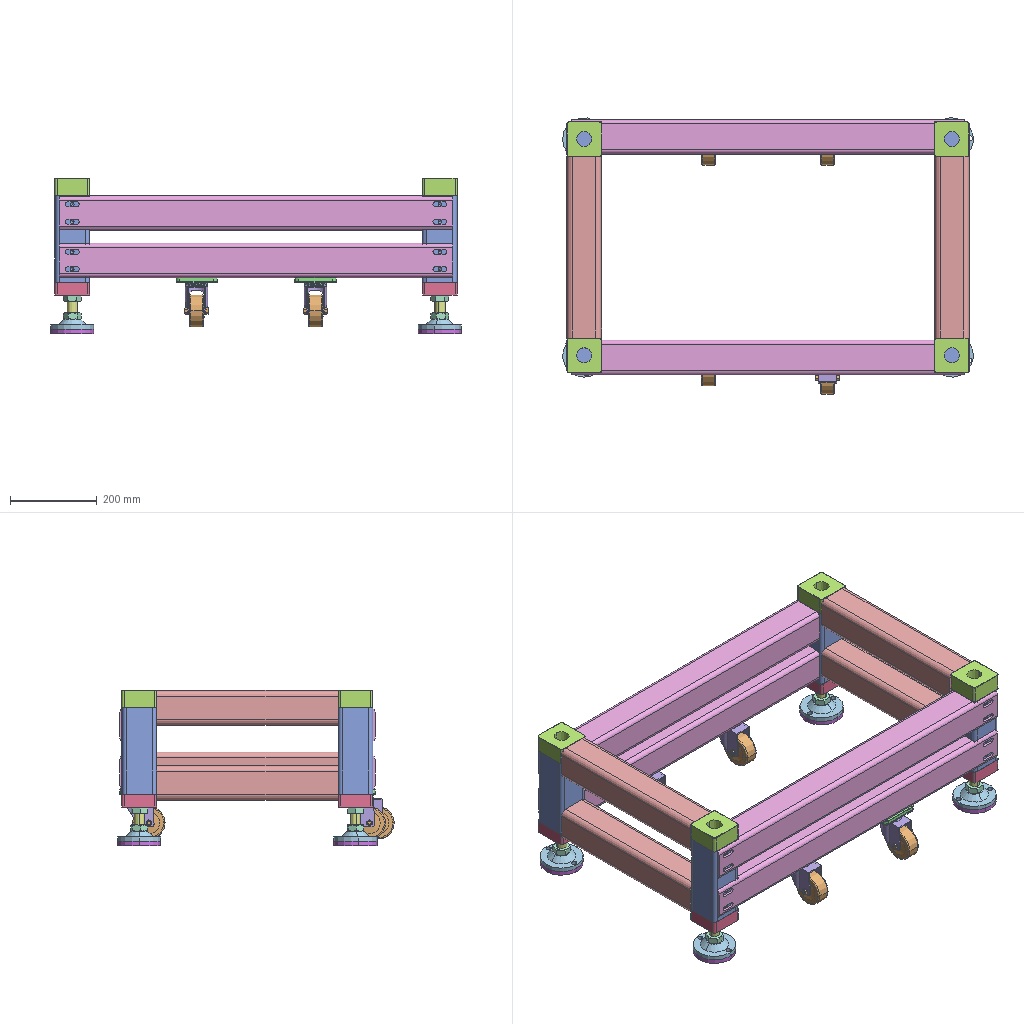Assembly | SolidWorks | 9 different items | 40 placed | box 950 x 639 x 359 mm
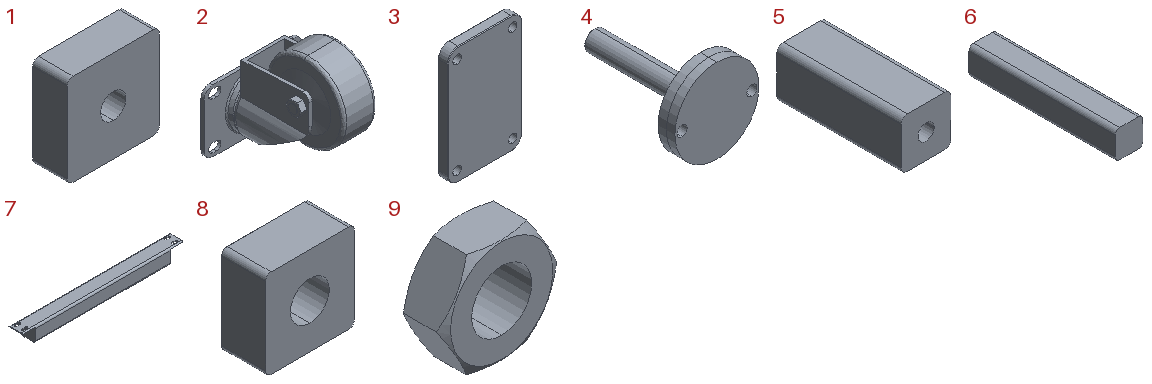Parts list (item | quantity | size | volume | features):
1 | x4 | 80 x 30 x 80 mm | 179952 mm3 | features Extrusion 1, Fillet 1, HoleWzd 1
2 | x4 | 95 x 106 x 104.5 mm | 205443 mm3 | features ICE 4, BaseBody 2, Fillet 2, Extrusion 1, Revolution 1
3 | x4 | 60 x 8 x 95 mm | 43868 mm3 | features Chamfer 1, Extrusion 1, Fillet 1, HoleWzd 1
4 | x4 | 100 x 146 x 100 mm | 232661 mm3 | features BaseBody 3
5 | x4 | 80 x 199.7 x 80 mm | 1203112 mm3 | features HoleWzd 2, Extrusion 1, Fillet 1, ICE 1
6 | x4 | 80 x 420 x 80 mm | 2623906 mm3 | features Extrusion 1
7 | x4 | 910 x 80 x 80 mm | 4905439 mm3 | features ICE 3, Extrusion 1, Fillet 1
8 | x4 | 80 x 40 x 80 mm | 216618 mm3 | features Chamfer 1, Extrusion 1, Fillet 1, HoleWzd 1
9 | x8 | 41.569 x 15 x 36.009 mm | 11607 mm3 | features Extrusion 1, RevCut 1
Mates (type | each side: item.copy, entity, surface, feature):
Parallel | 5.1 face plane Boss-Extrude1 | 8.1 face plane Boss-Extrude1 | 2 times
Coincident | 5.1 face plane Boss-Extrude1 | 8.1 face plane Boss-Extrude1 | 3 times
Parallel | 6.1 face plane Boss-Extrude1 | 8.2 face plane Boss-Extrude1 | 2 times
Coincident | 6.1 face plane Boss-Extrude1 | 8.2 face plane Boss-Extrude1 | 3 times
Parallel | 6.1 face plane Boss-Extrude1 | 8.1 face plane Boss-Extrude1
Coincident | 6.1 face plane Boss-Extrude1 | 8.1 face plane Boss-Extrude1 | 2 times
Coincident | 6.1 face plane Boss-Extrude1 | 5.1 face plane Boss-Extrude1
Parallel | 6.1 face plane Boss-Extrude1 | 6.2 face plane Boss-Extrude1
Coincident | 5.1 face plane Boss-Extrude1 | 6.2 face plane Boss-Extrude1
Coincident | 8.2 face plane Boss-Extrude1 | 5.2 face plane Boss-Extrude1 | 3 times
Coincident | 6.1 face plane Boss-Extrude1 | 5.2 face plane Boss-Extrude1
Coincident | 6.2 face plane Boss-Extrude1 | 5.2 face plane Boss-Extrude1
Coincident | 6.3 face plane Boss-Extrude1 | 5.3 face plane Boss-Extrude1
Coincident | 8.3 face plane Boss-Extrude1 | 5.4 face plane Boss-Extrude1 | 3 times
Coincident | 6.3 face plane Boss-Extrude1 | 8.3 face plane Boss-Extrude1 | 2 times
Coincident | 6.3 face plane Boss-Extrude1 | 5.4 face plane Boss-Extrude1
Coincident | 6.4 face plane Boss-Extrude1 | 5.4 face plane Boss-Extrude1 | 2 times
Parallel | 6.1 face plane Boss-Extrude1 | 6.3 face plane Boss-Extrude1
Coincident | 5.2 face plane Boss-Extrude1 | 7.1 face plane Boss-Extrude3
Coincident | 5.2 edge | 7.1 edge
Coincident | 8.2 edge | 7.1 face plane Boss-Extrude1
Coincident | 5.4 face plane Boss-Extrude1 | 7.1 face plane Boss-Extrude2
Coincident | 5.4 face plane Boss-Extrude1 | 7.1 face plane Boss-Extrude1
Coincident | 8.3 edge | 7.1 edge
Coincident | 7.2 face plane Boss-Extrude2 | 5.1 face plane Boss-Extrude1
Coincident | 5.1 edge | 7.2 edge
Coincident | 8.1 edge | 7.2 edge
Coincident | 5.3 face plane Boss-Extrude1 | 8.4 face plane Boss-Extrude1 | 3 times
Coincident | 6.3 face plane Boss-Extrude1 | 8.4 face plane Boss-Extrude1 | 2 times
Coincident | 5.3 face plane Boss-Extrude1 | 7.3 face plane Boss-Extrude3
Coincident | 5.3 edge | 7.3 edge
DistanceDim | 7.3 edge | 5.3 edge
Coincident | 5.2 face plane Boss-Extrude1 | 7.4 face plane Boss-Extrude3
Coincident | 5.4 edge | 7.4 edge
DistanceDim | 7.4 edge | 5.4 edge
Coincident | 3.1 face plane Boss-Extrude1 | 2.1 face plane Boss-Extrude1
Concentric | 3.1 edge | 2.1 edge | 2 times
Coincident | 3.2 face plane Boss-Extrude1 | 2.2 face plane Boss-Extrude1
Concentric | 3.2 face cylinder Ø6.8 (6.8) Diameter Hole1 | 2.2 edge
Concentric | 3.2 edge | 2.2 edge
Coincident | 2.3 face plane Boss-Extrude1 | 3.3 face plane Boss-Extrude1
Concentric | 2.3 edge | 3.3 edge
Concentric | 2.3 edge | 3.3 face cylinder Ø6.8 (6.8) Diameter Hole1
Coincident | 7.4 face plane Boss-Extrude1 | 3.2 face plane Boss-Extrude1 | 2 times
Coincident | 7.4 face plane Boss-Extrude1 | 3.1 face plane Boss-Extrude1 | 2 times
Coincident | 7.3 face plane Boss-Extrude1 | 3.3 face plane Boss-Extrude1 | 2 times
Coincident | 3.4 face plane Boss-Extrude1 | 2.4 face plane Boss-Extrude1
Concentric | 3.4 edge | 2.4 edge | 2 times
Coincident | 7.3 face plane Boss-Extrude1 | 3.4 face plane Boss-Extrude1 | 2 times
Coincident | 3.2 face plane Boss-Extrude1 | 3.4 face plane Boss-Extrude1
Coincident | 3.3 face plane Boss-Extrude1 | 3.1 face plane Boss-Extrude1
Coincident | 5.3 face plane Boss-Extrude1 | 1.1 face plane Boss-Extrude1 | 3 times
Concentric | 5.4 edge | 1.2 edge
Coincident | 5.4 face plane Boss-Extrude1 | 1.2 face plane Boss-Extrude1 | 2 times
Coincident | 5.1 face plane Boss-Extrude1 | 1.3 face plane Boss-Extrude1 | 3 times
Coincident | 5.2 face plane Boss-Extrude1 | 1.4 face plane Boss-Extrude1 | 3 times
Concentric | 1.2 edge | 4.1 face cylinder Input4
Concentric | 1.1 edge | 4.2 face cylinder Input4
Concentric | 1.4 edge | 4.3 face cylinder Input4
Concentric | 1.3 edge | 4.4 face cylinder Input4
DistanceDim | 1.1 face plane Boss-Extrude1 | 4.2 face plane Input5
Coincident | 4.2 face plane Input5 | 4.1 face plane Input5
Coincident | 4.4 face plane Input5 | 4.2 face plane Input5
Coincident | 4.4 face plane Input5 | 4.3 face plane Input5
DistanceDim | 1.3 face plane Boss-Extrude1 | 3.4 face plane Boss-Extrude1
DistanceDim | 3.3 face plane Boss-Extrude1 | 1.1 face plane Boss-Extrude1
Concentric | 4.1 face cylinder Input4 | 9.1 edge
Concentric | 4.1 face cylinder Input4 | 9.2 face cylinder Boss-Extrude1
Concentric | 4.2 face cylinder Input4 | 9.3 face cylinder Boss-Extrude1
Concentric | 4.2 face cylinder Input4 | 9.4 edge
Coincident | 1.1 face plane Boss-Extrude1 | 9.3 face plane Boss-Extrude1
Coincident | 4.2 face plane Input1 | 9.4 face plane Boss-Extrude1
Coincident | 1.2 face plane Boss-Extrude1 | 9.2 face plane Boss-Extrude1
Coincident | 4.1 face plane Input1 | 9.1 face plane Boss-Extrude1
Concentric | 4.4 face cylinder Input4 | 9.5 edge
Concentric | 4.4 face cylinder Input4 | 9.6 face cylinder Boss-Extrude1
Coincident | 1.3 face plane Boss-Extrude1 | 9.5 face plane Boss-Extrude1
Coincident | 4.4 face plane Input1 | 9.6 face plane Boss-Extrude1
Concentric | 4.3 face cylinder Input4 | 9.7 face cylinder Boss-Extrude1
Concentric | 4.3 face cylinder Input4 | 9.8 edge
Coincident | 4.3 face plane Input1 | 9.7 face plane Boss-Extrude1
Coincident | 1.4 face plane Boss-Extrude1 | 9.8 face plane Boss-Extrude1